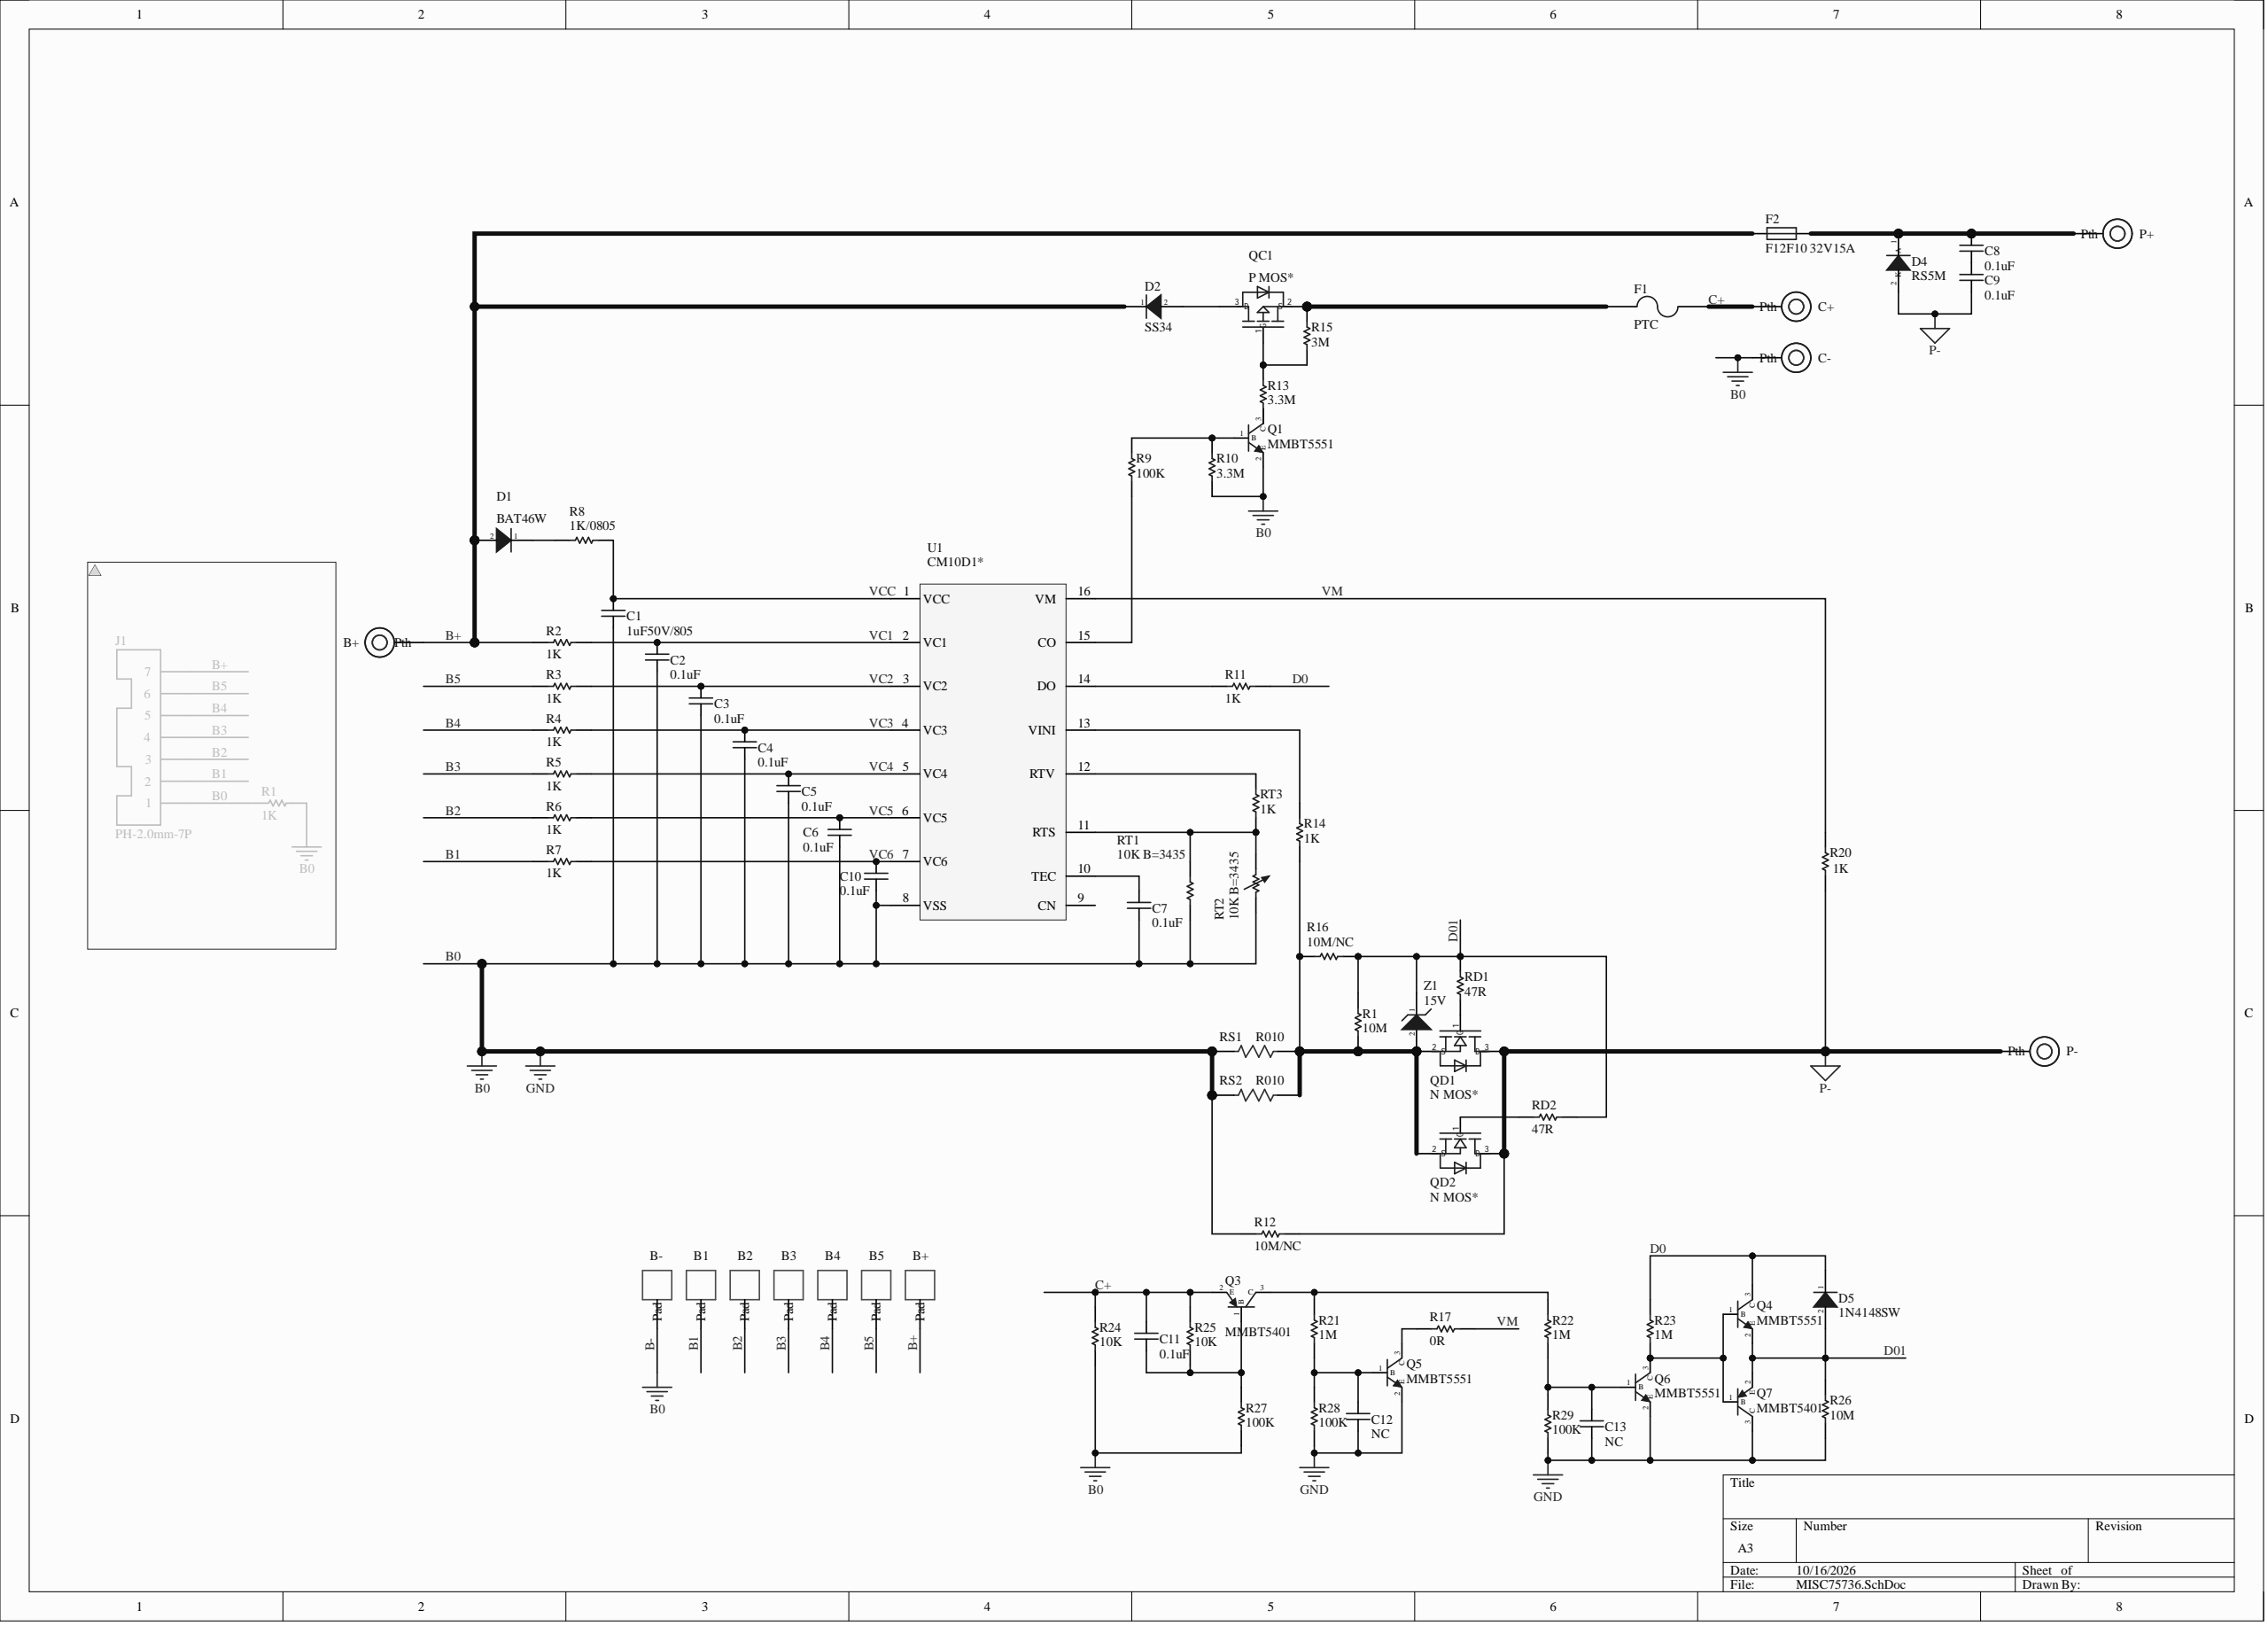Circuit board | Altium Designer | 76 parts | 42 nets
Bill of materials:
Comment,Description,Designator,Footprint,LibRef,Quantity
"Pad","connection pad (non-through-hole)","B1, B2, B3, B4, B5, B-, B+","Pad10X8mm","Pad","7"
"Pth","through-hole pad","B+, C-, C+, P-, P+","4*3","Pth","5"
"1uF50V/805","chip capacitor","C1","C0805L","CAP","1"
"0.1uF","chip capacitor","C2, C3, C4, C5, C6, C7, C8, C9, C10, C11","C0603A","CAP","10"
"NC","chip capacitor","C12, C13","C0603A","CAP","2"
"BAT46W","chip diode","D1","SOD323","BAT46W","1"
"SS34","chip Schottky diode","D2","SMB(DO-214AA)","SS34","1"
"RS5M","chip diode","D4","SMC A(DO-214AB)","RS5M","1"
"1N4148SW","chip diode","D5","SOD323","1N4148SW","1"
"PTC","chip resettable fuse","F1","F1812A","PTC","1"
"F12F10 32V15A","","F2","R1206A","FUSE","1"
"MMBT5551","chip transistor","Q1, Q4, Q5, Q6","SOT23-3","MMBT5551","4"
"MMBT5401","chip transistor","Q3, Q7","SOT23-3","MMBT5401","2"
"P MOS*","chip MOSFET","QC1","SOP-8L(T3p)","P MOS*","1"
"N MOS*","chip MOSFET","QD1, QD2","TO-252","N MOS*","2"
"10M","chip resistor","R1, R26","R0603A","RES","2"
"1K","chip resistor","R2, R3, R4, R5, R6, R7, R11, R14, R20, RT3","R0603A","RES","10"
"1K/0805","chip resistor","R8","R0805L","RES","1"
"100K","chip resistor","R9, R27, R28, R29","R0603A","RES","4"
"3.3M","chip resistor","R10, R13","R0603A","RES","2"
"10M/NC","chip resistor","R12, R16","R0603A","RES","2"
"3M","chip resistor","R15","R0603A","RES","1"
"0R","chip resistor","R17","R0603A","RES","1"
"1M","chip resistor","R21, R22, R23","R0603A","RES","3"
"10K","chip resistor","R24, R25","R0603A","RES","2"
"47R","chip resistor","RD1, RD2","R0603A","RES","2"
"R010","chip metal alloy resistor","RS1, RS2","R2512L","RES2","2"
"10K B=3435","chip resistor, chip thermistor","RT1, RT2","R0603A","RES, NTC","2"
"CM10D1*","6-cell battery protection IC","U1","SOP16L","CM1061*","1"
"15V","chip Zener diode","Z1","SOD323","15V","1"
Netlist (Protel format):
[
B1
Pad10X8mm
Pad



]
[
B2
Pad10X8mm
Pad



]
[
B3
Pad10X8mm
Pad



]
[
B4
Pad10X8mm
Pad



]
[
B5
Pad10X8mm
Pad



]
[
B+
Pad10X8mm
Pad



]
[
B+
4*3
Pth



]
[
B-
Pad10X8mm
Pad



]
[
C1
C0805L
1uF50V/805



]
[
C2
C0603A
0.1uF



]
[
C3
C0603A
0.1uF



]
[
C4
C0603A
0.1uF



]
[
C5
C0603A
0.1uF



]
[
C6
C0603A
0.1uF



]
[
C7
C0603A
0.1uF



]
[
C8
C0603A
0.1uF



]
[
C9
C0603A
0.1uF



]
[
C10
C0603A
0.1uF



]
[
C11
C0603A
0.1uF



]
[
C12
C0603A
NC



]
[
C13
C0603A
NC



]
[
C+
4*3
Pth



]
[
C-
4*3
Pth



]
[
D1
SOD323
BAT46W



]
[
D2
SMB(DO-214AA)
SS34



]
[
D4
SMC A(DO-214AB)
RS5M



]
[
D5
SOD323
1N4148SW



]
[
F1
F1812A
PTC



]
[
F2
R1206A
F12F10 32V15A



]
[
P+
4*3
Pth



]
[
P-
4*3
Pth



]
[
Q1
SOT23-3
MMBT5551



]
[
Q3
SOT23-3
MMBT5401



]
[
Q4
SOT23-3
MMBT5551



]
[
Q5
SOT23-3
MMBT5551



]
[
Q6
SOT23-3
MMBT5551



]
[
Q7
SOT23-3
MMBT5401



]
[
QC1
SOP-8L(T3p)
P MOS*



]
[
QD1
TO-252
N MOS*



]
[
QD2
TO-252
N MOS*



]
[
R1
R0603A
10M



]
[
R2
R0603A
1K



]
[
R3
R0603A
1K



]
[
R4
R0603A
1K



]
[
R5
R0603A
1K



]
[
R6
R0603A
1K



]
[
R7
R0603A
1K



]
[
R8
R0805L
1K/0805



]
[
R9
R0603A
100K



]
[
R10
R0603A
3.3M



]
[
R11
R0603A
1K



]
[
R12
R0603A
10M/NC



]
[
R13
R0603A
3.3M



]
[
R14
R0603A
1K



]
[
R15
R0603A
3M



]
[
R16
R0603A
10M/NC



]
[
R17
R0603A
0R



]
[
R20
R0603A
1K



]
[
R21
R0603A
1M



]
[
R22
R0603A
1M



]
[
R23
R0603A
1M



]
[
R24
R0603A
10K



]
[
R25
R0603A
10K



]
[
R26
R0603A
10M



]
[
R27
R0603A
100K



]
[
R28
R0603A
100K



]
[
R29
R0603A
100K



]
[
RD1
R0603A
47R



]
[
RD2
R0603A
47R



]
[
RS1
R2512L
R010



]
[
RS2
R2512L
R010



]
[
RT1
R0603A
10K B=3435



]
[
RT2
R0603A
10K B=3435



]
[
RT3
R0603A
1K



]
[
U1
SOP16L
CM10D1*



]
[
Z1
SOD323
15V



]
(
VM
R17-1
R20-2
U1-16
)
(
VCC
C1-2
R8-2
U1-1
)
(
VC6
C10-2
R7-2
U1-7
)
(
VC5
C6-2
R6-2
U1-6
)
(
VC4
C5-2
R5-2
U1-5
)
(
VC3
C4-2
R4-2
U1-4
)
(
VC2
C3-2
R3-2
U1-3
)
(
VC1
C2-2
R2-2
U1-2
)
(
P-
C9-2
D4-2
P--1
QD1-3
QD2-3
R12-2
R20-1
)
(
NetRT3_2
RT3-2
U1-12
)
(
NetRT1_2
RT1-2
RT2-2
RT3-1
U1-11
)
(
NetR14_2
R14-2
U1-13
)
(
NetR11_2
R11-2
U1-14
)
(
NetR9_1
R9-1
U1-15
)
(
NetQD2_1
QD2-1
RD2-1
)
(
NetQD1_2
QD1-2
QD2-2
R1-1
R14-1
R16-1
RS1-2
RS2-2
Z1-2
)
(
NetQD1_1
QD1-1
RD1-2
)
(
NetQC1_1
QC1-1
R13-2
R15-1
)
(
NetQ5_3
Q5-3
R17-2
)
(
NetQ4_1
Q4-1
Q6-3
Q7-1
R23-1
)
(
NetQ3_3
Q3-3
R21-2
R22-2
)
(
NetQ1_3
Q1-3
R13-1
)
(
NetQ1_1
Q1-1
R9-2
R10-2
)
(
NetF1_1
F1-1
QC1-2
R15-2
)
(
NetD2_2
D2-2
QC1-3
)
(
NetD1_1
D1-1
R8-1
)
(
NetC13_1
C13-1
Q6-1
R22-1
R29-2
)
(
NetC12_1
C12-1
Q5-1
R21-1
R28-2
)
(
NetC11_2
C11-2
Q3-1
R25-1
R27-2
)
(
NetC8_2
C8-2
C9-1
)
(
NetC8_1
C8-1
D4-1
F2-2
P+-1
)
(
NetC7_1
C7-1
U1-10
)
(
D01
D5-2
Q4-2
Q7-2
R1-2
R16-2
R26-2
RD1-1
RD2-2
Z1-1
)
(
D0
D5-1
Q4-3
R11-1
R23-2
)
(
C+
C11-1
C+-1
F1-2
Q3-2
R24-2
R25-2
)
(
B+
B+-1
B+-1
D1-2
D2-1
F2-1
R2-1
)
(
B5
B5-1
R3-1
)
(
B4
B4-1
R4-1
)
(
B3
B3-1
R5-1
)
(
B2
B2-1
R6-1
)
(
B1
B1-1
R7-1
)
(
B0
B--1
C1-1
C2-1
C3-1
C4-1
C5-1
C6-1
C7-2
C10-1
C12-2
C13-2
C--1
Q1-2
Q5-2
Q6-2
Q7-3
R10-1
R12-1
R24-1
R26-1
R27-1
R28-1
R29-1
RS1-1
RS2-1
RT1-1
RT2-1
U1-8
)